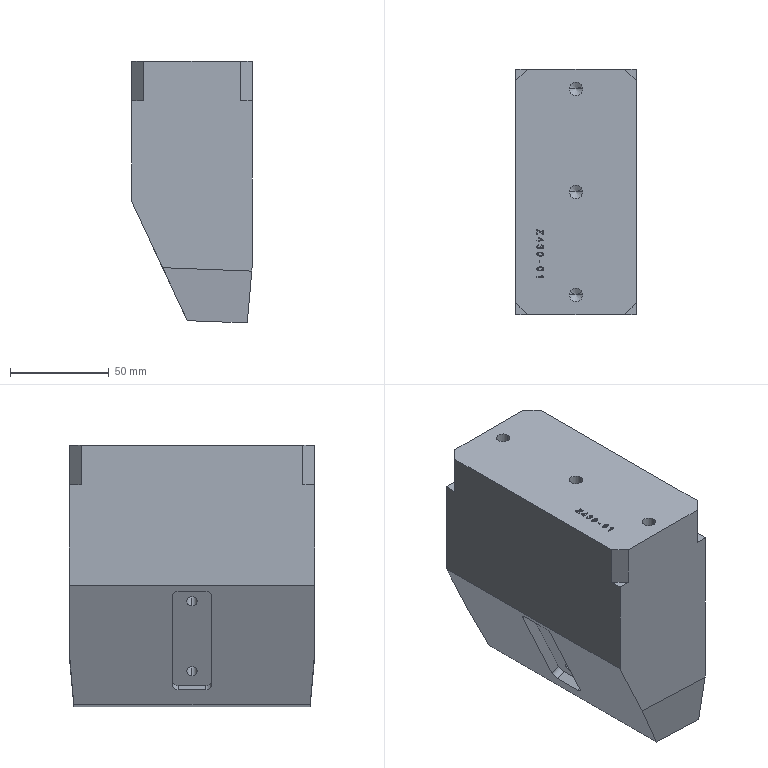Part | Creo | 1 solid | 166 faces | box 61 x 124 x 132.313 mm | volume 872756 mm3 | other 79 | plane 62 | cylinder 15 | cone 10 | commonest cylinder face diameters 6.8 x6 5.1 x4 6 x4 45.582 x1